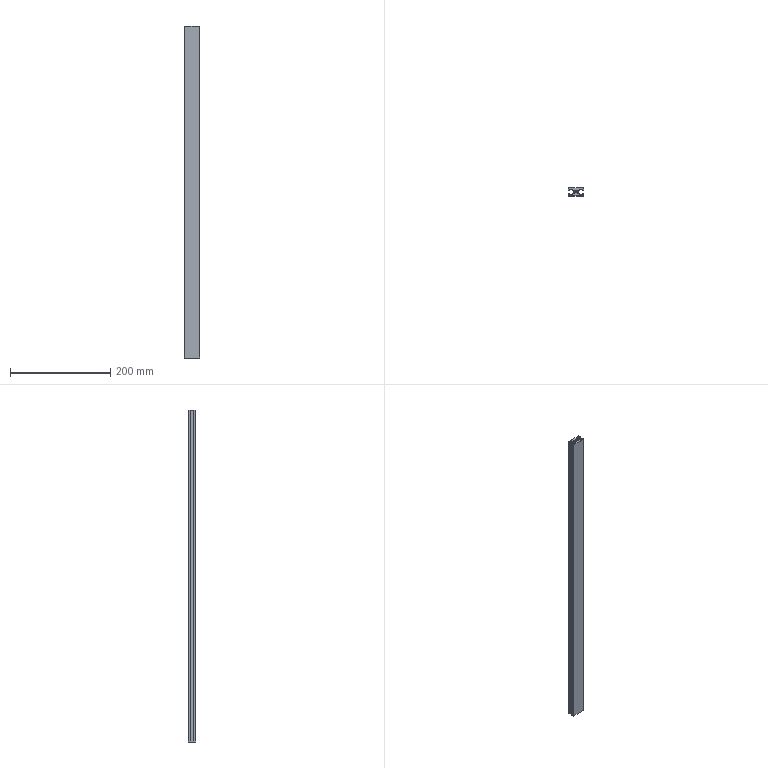Part | SolidWorks | features BaseBody 1, HoleWzd 1, MoveFace 1 | 1 solid | 85 faces | box 30 x 15 x 662 mm | volume 159462 mm3 | cylinder 39 | plane 38 | cone 8 | commonest cylinder face diameters 3.3 x16 5 x13 1 x6 2 x4